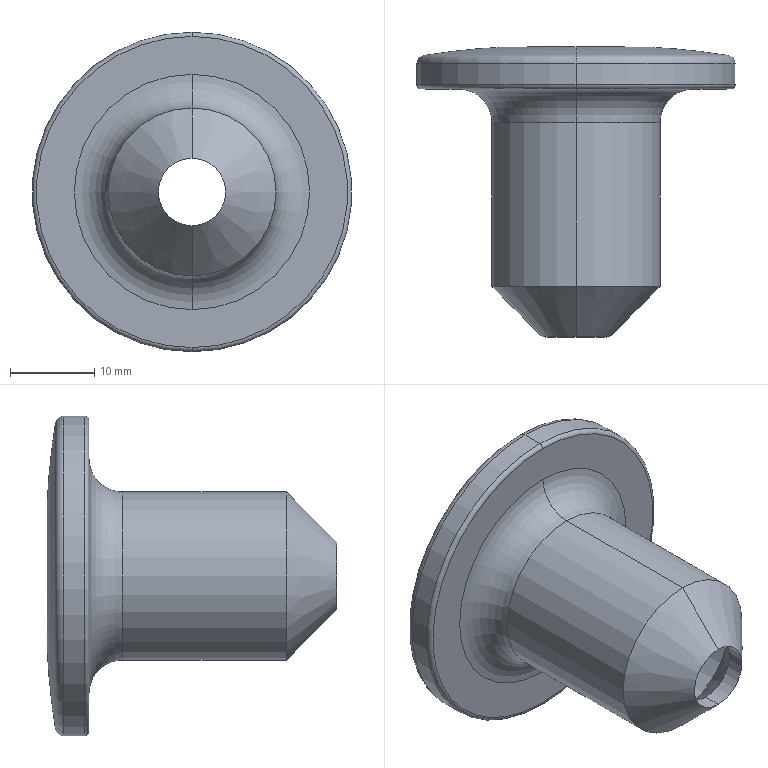Part | SolidWorks | features Cut 1, ICE 1, Revolution 1 | 1 solid | 27 faces | box 38 x 34.477 x 38 mm | volume 6932 mm3 | cylinder 12 | torus 8 | cone 4 | plane 3 | commonest cylinder face diameters 17 x4 8 x2 11 x2 20 x2 38 x2
STEP:
#1=CARTESIAN_POINT('',(0.,-17.379,-4.));
#2=VERTEX_POINT('',#1);
#3=CARTESIAN_POINT('',(0.,-17.379,4.));
#4=VERTEX_POINT('',#3);
#5=CARTESIAN_POINT('',(0.,-17.379,0.));
#6=DIRECTION('',(0.,1.,0.));
#7=DIRECTION('',(0.,0.,1.));
#8=AXIS2_PLACEMENT_3D('',#5,#6,#7);
#9=CIRCLE('',#8,4.);
#10=EDGE_CURVE('',#2,#4,#9,.T.);
#11=ORIENTED_EDGE('',*,*,#10,.T.);
#12=CARTESIAN_POINT('',(0.,-19.5,4.));
#13=VERTEX_POINT('',#12);
#14=CARTESIAN_POINT('',(0.,-10.,4.));
#15=DIRECTION('',(0.,-1.,0.));
#16=VECTOR('',#15,1000.);
#17=LINE('',#14,#16);
#18=EDGE_CURVE('',#4,#13,#17,.T.);
#19=ORIENTED_EDGE('',*,*,#18,.T.);
#20=CARTESIAN_POINT('',(0.,-19.5,-4.));
#21=VERTEX_POINT('',#20);
#22=CARTESIAN_POINT('',(0.,-19.5,0.));
#23=DIRECTION('',(0.,1.,0.));
#24=DIRECTION('',(0.,0.,1.));
#25=AXIS2_PLACEMENT_3D('',#22,#23,#24);
#26=CIRCLE('',#25,4.);
#27=EDGE_CURVE('',#21,#13,#26,.T.);
#28=ORIENTED_EDGE('',*,*,#27,.F.);
#29=CARTESIAN_POINT('',(0.,-10.,-4.));
#30=DIRECTION('',(0.,-1.,0.));
#31=VECTOR('',#30,1000.);
#32=LINE('',#29,#31);
#33=EDGE_CURVE('',#2,#21,#32,.T.);
#34=ORIENTED_EDGE('',*,*,#33,.F.);
#35=EDGE_LOOP('',(#11,#19,#28,#34));
#36=FACE_OUTER_BOUND('',#35,.T.);
#37=CARTESIAN_POINT('',(0.,-10.,0.));
#38=DIRECTION('',(0.,-1.,0.));
#39=DIRECTION('',(0.,0.,-1.));
#40=AXIS2_PLACEMENT_3D('',#37,#38,#39);
#41=CYLINDRICAL_SURFACE('',#40,4.);
#42=ADVANCED_FACE('',(#36),#41,.F.);
#43=CARTESIAN_POINT('',(0.,10.5,19.));
#44=VERTEX_POINT('',#43);
#45=CARTESIAN_POINT('',(0.,10.5,-19.));
#46=VERTEX_POINT('',#45);
#47=CARTESIAN_POINT('',(0.,10.5,0.));
#48=DIRECTION('',(0.,1.,0.));
#49=DIRECTION('',(0.,0.,1.));
#50=AXIS2_PLACEMENT_3D('',#47,#48,#49);
#51=CIRCLE('',#50,19.);
#52=EDGE_CURVE('',#44,#46,#51,.T.);
#53=ORIENTED_EDGE('',*,*,#52,.T.);
#54=CARTESIAN_POINT('',(0.,13.,-19.));
#55=VERTEX_POINT('',#54);
#56=CARTESIAN_POINT('',(0.,14.,-19.));
#57=DIRECTION('',(0.,1.,0.));
#58=VECTOR('',#57,1000.);
#59=LINE('',#56,#58);
#60=EDGE_CURVE('',#46,#55,#59,.T.);
#61=ORIENTED_EDGE('',*,*,#60,.T.);
#62=CARTESIAN_POINT('',(0.,13.,19.));
#63=VERTEX_POINT('',#62);
#64=CARTESIAN_POINT('',(0.,13.,0.));
#65=DIRECTION('',(0.,1.,0.));
#66=DIRECTION('',(0.,0.,1.));
#67=AXIS2_PLACEMENT_3D('',#64,#65,#66);
#68=CIRCLE('',#67,19.);
#69=EDGE_CURVE('',#63,#55,#68,.T.);
#70=ORIENTED_EDGE('',*,*,#69,.F.);
#71=CARTESIAN_POINT('',(0.,14.,19.));
#72=DIRECTION('',(0.,1.,0.));
#73=VECTOR('',#72,1000.);
#74=LINE('',#71,#73);
#75=EDGE_CURVE('',#44,#63,#74,.T.);
#76=ORIENTED_EDGE('',*,*,#75,.F.);
#77=EDGE_LOOP('',(#53,#61,#70,#76));
#78=FACE_OUTER_BOUND('',#77,.T.);
#79=CARTESIAN_POINT('',(0.,14.,0.));
#80=DIRECTION('',(0.,1.,0.));
#81=DIRECTION('',(0.,0.,1.));
#82=AXIS2_PLACEMENT_3D('',#79,#80,#81);
#83=CYLINDRICAL_SURFACE('',#82,19.);
#84=ADVANCED_FACE('',(#78),#83,.T.);
#85=ORIENTED_EDGE('',*,*,#69,.T.);
#86=CARTESIAN_POINT('',(0.,14.,-18.));
#87=VERTEX_POINT('',#86);
#88=CARTESIAN_POINT('',(0.,13.,-18.));
#89=DIRECTION('',(1.,0.,0.));
#90=DIRECTION('',(0.,0.,-1.));
#91=AXIS2_PLACEMENT_3D('',#88,#89,#90);
#92=CIRCLE('',#91,1.);
#93=EDGE_CURVE('',#55,#87,#92,.T.);
#94=ORIENTED_EDGE('',*,*,#93,.T.);
#95=CARTESIAN_POINT('',(0.,14.,18.));
#96=VERTEX_POINT('',#95);
#97=CARTESIAN_POINT('',(0.,14.,0.));
#98=DIRECTION('',(0.,1.,0.));
#99=DIRECTION('',(0.,0.,1.));
#100=AXIS2_PLACEMENT_3D('',#97,#98,#99);
#101=CIRCLE('',#100,18.);
#102=EDGE_CURVE('',#96,#87,#101,.T.);
#103=ORIENTED_EDGE('',*,*,#102,.F.);
#104=CARTESIAN_POINT('',(0.,13.,18.));
#105=DIRECTION('',(-1.,0.,0.));
#106=DIRECTION('',(0.,0.,1.));
#107=AXIS2_PLACEMENT_3D('',#104,#105,#106);
#108=CIRCLE('',#107,1.);
#109=EDGE_CURVE('',#63,#96,#108,.T.);
#110=ORIENTED_EDGE('',*,*,#109,.F.);
#111=EDGE_LOOP('',(#85,#94,#103,#110));
#112=FACE_OUTER_BOUND('',#111,.T.);
#113=CARTESIAN_POINT('',(0.,13.,0.));
#114=DIRECTION('',(0.,1.,0.));
#115=DIRECTION('',(0.,0.,1.));
#116=AXIS2_PLACEMENT_3D('',#113,#114,#115);
#117=TOROIDAL_SURFACE('',#116,18.,1.);
#118=ADVANCED_FACE('',(#112),#117,.T.);
#119=ORIENTED_EDGE('',*,*,#102,.T.);
#120=CARTESIAN_POINT('',(0.,14.977,-8.5));
#121=VERTEX_POINT('',#120);
#122=CARTESIAN_POINT('',(0.,-66.038,-4.966));
#123=DIRECTION('',(1.,0.,0.));
#124=DIRECTION('',(0.,0.,-1.));
#125=AXIS2_PLACEMENT_3D('',#122,#123,#124);
#126=CIRCLE('',#125,81.092);
#127=EDGE_CURVE('',#87,#121,#126,.T.);
#128=ORIENTED_EDGE('',*,*,#127,.T.);
#129=CARTESIAN_POINT('',(0.,14.977,8.5));
#130=VERTEX_POINT('',#129);
#131=CARTESIAN_POINT('',(0.,14.977,0.));
#132=DIRECTION('',(0.,1.,0.));
#133=DIRECTION('',(0.,0.,1.));
#134=AXIS2_PLACEMENT_3D('',#131,#132,#133);
#135=CIRCLE('',#134,8.5);
#136=EDGE_CURVE('',#130,#121,#135,.T.);
#137=ORIENTED_EDGE('',*,*,#136,.F.);
#138=CARTESIAN_POINT('',(0.,-66.038,4.966));
#139=DIRECTION('',(-1.,0.,0.));
#140=DIRECTION('',(0.,0.,1.));
#141=AXIS2_PLACEMENT_3D('',#138,#139,#140);
#142=CIRCLE('',#141,81.092);
#143=EDGE_CURVE('',#96,#130,#142,.T.);
#144=ORIENTED_EDGE('',*,*,#143,.F.);
#145=EDGE_LOOP('',(#119,#128,#137,#144));
#146=FACE_OUTER_BOUND('',#145,.T.);
#147=CARTESIAN_POINT('',(0.,-66.038,0.));
#148=DIRECTION('',(0.,1.,0.));
#149=DIRECTION('',(0.,0.,1.));
#150=AXIS2_PLACEMENT_3D('',#147,#148,#149);
#151=TOROIDAL_SURFACE('',#150,4.966,81.092);
#152=ADVANCED_FACE('',(#146),#151,.T.);
#153=CARTESIAN_POINT('',(0.,5.,-8.5));
#154=VERTEX_POINT('',#153);
#155=CARTESIAN_POINT('',(0.,5.,8.5));
#156=VERTEX_POINT('',#155);
#157=CARTESIAN_POINT('',(0.,5.,0.));
#158=DIRECTION('',(0.,1.,0.));
#159=DIRECTION('',(0.,0.,1.));
#160=AXIS2_PLACEMENT_3D('',#157,#158,#159);
#161=CIRCLE('',#160,8.5);
#162=EDGE_CURVE('',#154,#156,#161,.T.);
#163=ORIENTED_EDGE('',*,*,#162,.F.);
#164=CARTESIAN_POINT('',(0.,14.,-8.5));
#165=DIRECTION('',(0.,1.,0.));
#166=VECTOR('',#165,1000.);
#167=LINE('',#164,#166);
#168=EDGE_CURVE('',#154,#121,#167,.T.);
#169=ORIENTED_EDGE('',*,*,#168,.T.);
#170=CARTESIAN_POINT('',(0.,14.977,0.));
#171=DIRECTION('',(0.,1.,0.));
#172=DIRECTION('',(0.,0.,1.));
#173=AXIS2_PLACEMENT_3D('',#170,#171,#172);
#174=CIRCLE('',#173,8.5);
#175=EDGE_CURVE('',#121,#130,#174,.T.);
#176=ORIENTED_EDGE('',*,*,#175,.T.);
#177=CARTESIAN_POINT('',(0.,14.,8.5));
#178=DIRECTION('',(0.,1.,0.));
#179=VECTOR('',#178,1000.);
#180=LINE('',#177,#179);
#181=EDGE_CURVE('',#156,#130,#180,.T.);
#182=ORIENTED_EDGE('',*,*,#181,.F.);
#183=EDGE_LOOP('',(#163,#169,#176,#182));
#184=FACE_OUTER_BOUND('',#183,.T.);
#185=CARTESIAN_POINT('',(0.,14.,0.));
#186=DIRECTION('',(0.,1.,0.));
#187=DIRECTION('',(0.,0.,1.));
#188=AXIS2_PLACEMENT_3D('',#185,#186,#187);
#189=CYLINDRICAL_SURFACE('',#188,8.5);
#190=ADVANCED_FACE('',(#184),#189,.F.);
#191=CARTESIAN_POINT('',(0.,3.5,-5.5));
#192=VERTEX_POINT('',#191);
#193=CARTESIAN_POINT('',(0.,3.5,5.5));
#194=VERTEX_POINT('',#193);
#195=CARTESIAN_POINT('',(0.,3.5,0.));
#196=DIRECTION('',(0.,1.,0.));
#197=DIRECTION('',(0.,0.,1.));
#198=AXIS2_PLACEMENT_3D('',#195,#196,#197);
#199=CIRCLE('',#198,5.5);
#200=EDGE_CURVE('',#192,#194,#199,.T.);
#201=ORIENTED_EDGE('',*,*,#200,.F.);
#202=CARTESIAN_POINT('',(0.,5.,-5.5));
#203=VERTEX_POINT('',#202);
#204=CARTESIAN_POINT('',(0.,14.,-5.5));
#205=DIRECTION('',(0.,1.,0.));
#206=VECTOR('',#205,1000.);
#207=LINE('',#204,#206);
#208=EDGE_CURVE('',#192,#203,#207,.T.);
#209=ORIENTED_EDGE('',*,*,#208,.T.);
#210=CARTESIAN_POINT('',(0.,5.,5.5));
#211=VERTEX_POINT('',#210);
#212=CARTESIAN_POINT('',(0.,5.,0.));
#213=DIRECTION('',(0.,1.,0.));
#214=DIRECTION('',(0.,0.,1.));
#215=AXIS2_PLACEMENT_3D('',#212,#213,#214);
#216=CIRCLE('',#215,5.5);
#217=EDGE_CURVE('',#203,#211,#216,.T.);
#218=ORIENTED_EDGE('',*,*,#217,.T.);
#219=CARTESIAN_POINT('',(0.,14.,5.5));
#220=DIRECTION('',(0.,1.,0.));
#221=VECTOR('',#220,1000.);
#222=LINE('',#219,#221);
#223=EDGE_CURVE('',#194,#211,#222,.T.);
#224=ORIENTED_EDGE('',*,*,#223,.F.);
#225=EDGE_LOOP('',(#201,#209,#218,#224));
#226=FACE_OUTER_BOUND('',#225,.T.);
#227=CARTESIAN_POINT('',(0.,14.,0.));
#228=DIRECTION('',(0.,1.,0.));
#229=DIRECTION('',(0.,0.,1.));
#230=AXIS2_PLACEMENT_3D('',#227,#228,#229);
#231=CYLINDRICAL_SURFACE('',#230,5.5);
#232=ADVANCED_FACE('',(#226),#231,.F.);
#233=CARTESIAN_POINT('',(0.,-12.879,-8.5));
#234=VERTEX_POINT('',#233);
#235=CARTESIAN_POINT('',(0.,-12.879,8.5));
#236=VERTEX_POINT('',#235);
#237=CARTESIAN_POINT('',(0.,-12.879,0.));
#238=DIRECTION('',(0.,1.,0.));
#239=DIRECTION('',(0.,0.,1.));
#240=AXIS2_PLACEMENT_3D('',#237,#238,#239);
#241=CIRCLE('',#240,8.5);
#242=EDGE_CURVE('',#234,#236,#241,.T.);
#243=ORIENTED_EDGE('',*,*,#242,.F.);
#244=CARTESIAN_POINT('',(0.,3.5,-8.5));
#245=VERTEX_POINT('',#244);
#246=CARTESIAN_POINT('',(0.,14.,-8.5));
#247=DIRECTION('',(0.,1.,0.));
#248=VECTOR('',#247,1000.);
#249=LINE('',#246,#248);
#250=EDGE_CURVE('',#234,#245,#249,.T.);
#251=ORIENTED_EDGE('',*,*,#250,.T.);
#252=CARTESIAN_POINT('',(0.,3.5,8.5));
#253=VERTEX_POINT('',#252);
#254=CARTESIAN_POINT('',(0.,3.5,0.));
#255=DIRECTION('',(0.,1.,0.));
#256=DIRECTION('',(0.,0.,1.));
#257=AXIS2_PLACEMENT_3D('',#254,#255,#256);
#258=CIRCLE('',#257,8.5);
#259=EDGE_CURVE('',#245,#253,#258,.T.);
#260=ORIENTED_EDGE('',*,*,#259,.T.);
#261=CARTESIAN_POINT('',(0.,14.,8.5));
#262=DIRECTION('',(0.,1.,0.));
#263=VECTOR('',#262,1000.);
#264=LINE('',#261,#263);
#265=EDGE_CURVE('',#236,#253,#264,.T.);
#266=ORIENTED_EDGE('',*,*,#265,.F.);
#267=EDGE_LOOP('',(#243,#251,#260,#266));
#268=FACE_OUTER_BOUND('',#267,.T.);
#269=CARTESIAN_POINT('',(0.,14.,0.));
#270=DIRECTION('',(0.,1.,0.));
#271=DIRECTION('',(0.,0.,1.));
#272=AXIS2_PLACEMENT_3D('',#269,#270,#271);
#273=CYLINDRICAL_SURFACE('',#272,8.5);
#274=ADVANCED_FACE('',(#268),#273,.F.);
#275=ORIENTED_EDGE('',*,*,#10,.F.);
#276=CARTESIAN_POINT('',(0.,-18.5,-2.879));
#277=DIRECTION('',(0.,0.7071,-0.7071));
#278=VECTOR('',#277,1000.);
#279=LINE('',#276,#278);
#280=EDGE_CURVE('',#2,#234,#279,.T.);
#281=ORIENTED_EDGE('',*,*,#280,.T.);
#282=ORIENTED_EDGE('',*,*,#242,.T.);
#283=CARTESIAN_POINT('',(0.,-18.5,2.879));
#284=DIRECTION('',(0.,0.7071,0.7071));
#285=VECTOR('',#284,1000.);
#286=LINE('',#283,#285);
#287=EDGE_CURVE('',#4,#236,#286,.T.);
#288=ORIENTED_EDGE('',*,*,#287,.F.);
#289=EDGE_LOOP('',(#275,#281,#282,#288));
#290=FACE_OUTER_BOUND('',#289,.T.);
#291=CARTESIAN_POINT('',(0.,-18.5,0.));
#292=DIRECTION('',(0.,1.,0.));
#293=DIRECTION('',(0.,0.,1.));
#294=AXIS2_PLACEMENT_3D('',#291,#292,#293);
#295=CONICAL_SURFACE('',#294,2.879,0.7854);
#296=ADVANCED_FACE('',(#290),#295,.F.);
#297=CARTESIAN_POINT('',(0.,-19.5,0.));
#298=DIRECTION('',(0.,1.,0.));
#299=DIRECTION('',(0.,0.,1.));
#300=AXIS2_PLACEMENT_3D('',#297,#298,#299);
#301=CIRCLE('',#300,4.);
#302=EDGE_CURVE('',#13,#21,#301,.T.);
#303=ORIENTED_EDGE('',*,*,#302,.T.);
#304=CARTESIAN_POINT('',(0.,-13.5,-10.));
#305=VERTEX_POINT('',#304);
#306=CARTESIAN_POINT('',(0.,-20.,-3.5));
#307=DIRECTION('',(0.,0.7071,-0.7071));
#308=VECTOR('',#307,1000.);
#309=LINE('',#306,#308);
#310=EDGE_CURVE('',#21,#305,#309,.T.);
#311=ORIENTED_EDGE('',*,*,#310,.T.);
#312=CARTESIAN_POINT('',(0.,-13.5,10.));
#313=VERTEX_POINT('',#312);
#314=CARTESIAN_POINT('',(0.,-13.5,0.));
#315=DIRECTION('',(0.,1.,0.));
#316=DIRECTION('',(0.,0.,1.));
#317=AXIS2_PLACEMENT_3D('',#314,#315,#316);
#318=CIRCLE('',#317,10.);
#319=EDGE_CURVE('',#313,#305,#318,.T.);
#320=ORIENTED_EDGE('',*,*,#319,.F.);
#321=CARTESIAN_POINT('',(0.,-20.,3.5));
#322=DIRECTION('',(0.,0.7071,0.7071));
#323=VECTOR('',#322,1000.);
#324=LINE('',#321,#323);
#325=EDGE_CURVE('',#13,#313,#324,.T.);
#326=ORIENTED_EDGE('',*,*,#325,.F.);
#327=EDGE_LOOP('',(#303,#311,#320,#326));
#328=FACE_OUTER_BOUND('',#327,.T.);
#329=CARTESIAN_POINT('',(0.,-20.,0.));
#330=DIRECTION('',(0.,1.,0.));
#331=DIRECTION('',(0.,0.,1.));
#332=AXIS2_PLACEMENT_3D('',#329,#330,#331);
#333=CONICAL_SURFACE('',#332,3.5,0.7854);
#334=ADVANCED_FACE('',(#328),#333,.T.);
#335=ORIENTED_EDGE('',*,*,#319,.T.);
#336=CARTESIAN_POINT('',(0.,6.,-10.));
#337=VERTEX_POINT('',#336);
#338=CARTESIAN_POINT('',(0.,14.,-10.));
#339=DIRECTION('',(0.,1.,0.));
#340=VECTOR('',#339,1000.);
#341=LINE('',#338,#340);
#342=EDGE_CURVE('',#305,#337,#341,.T.);
#343=ORIENTED_EDGE('',*,*,#342,.T.);
#344=CARTESIAN_POINT('',(0.,6.,10.));
#345=VERTEX_POINT('',#344);
#346=CARTESIAN_POINT('',(0.,6.,0.));
#347=DIRECTION('',(0.,1.,0.));
#348=DIRECTION('',(0.,0.,1.));
#349=AXIS2_PLACEMENT_3D('',#346,#347,#348);
#350=CIRCLE('',#349,10.);
#351=EDGE_CURVE('',#345,#337,#350,.T.);
#352=ORIENTED_EDGE('',*,*,#351,.F.);
#353=CARTESIAN_POINT('',(0.,14.,10.));
#354=DIRECTION('',(0.,1.,0.));
#355=VECTOR('',#354,1000.);
#356=LINE('',#353,#355);
#357=EDGE_CURVE('',#313,#345,#356,.T.);
#358=ORIENTED_EDGE('',*,*,#357,.F.);
#359=EDGE_LOOP('',(#335,#343,#352,#358));
#360=FACE_OUTER_BOUND('',#359,.T.);
#361=CARTESIAN_POINT('',(0.,14.,0.));
#362=DIRECTION('',(0.,1.,0.));
#363=DIRECTION('',(0.,0.,1.));
#364=AXIS2_PLACEMENT_3D('',#361,#362,#363);
#365=CYLINDRICAL_SURFACE('',#364,10.);
#366=ADVANCED_FACE('',(#360),#365,.T.);
#367=CARTESIAN_POINT('',(0.,10.,-14.));
#368=VERTEX_POINT('',#367);
#369=CARTESIAN_POINT('',(0.,10.,14.));
#370=VERTEX_POINT('',#369);
#371=CARTESIAN_POINT('',(0.,10.,0.));
#372=DIRECTION('',(0.,1.,0.));
#373=DIRECTION('',(0.,0.,1.));
#374=AXIS2_PLACEMENT_3D('',#371,#372,#373);
#375=CIRCLE('',#374,14.);
#376=EDGE_CURVE('',#368,#370,#375,.T.);
#377=ORIENTED_EDGE('',*,*,#376,.F.);
#378=CARTESIAN_POINT('',(0.,6.,-14.));
#379=DIRECTION('',(1.,0.,0.));
#380=DIRECTION('',(0.,0.,-1.));
#381=AXIS2_PLACEMENT_3D('',#378,#379,#380);
#382=CIRCLE('',#381,4.);
#383=EDGE_CURVE('',#368,#337,#382,.T.);
#384=ORIENTED_EDGE('',*,*,#383,.T.);
#385=CARTESIAN_POINT('',(0.,6.,0.));
#386=DIRECTION('',(0.,1.,0.));
#387=DIRECTION('',(0.,0.,1.));
#388=AXIS2_PLACEMENT_3D('',#385,#386,#387);
#389=CIRCLE('',#388,10.);
#390=EDGE_CURVE('',#337,#345,#389,.T.);
#391=ORIENTED_EDGE('',*,*,#390,.T.);
#392=CARTESIAN_POINT('',(0.,6.,14.));
#393=DIRECTION('',(-1.,0.,0.));
#394=DIRECTION('',(0.,0.,1.));
#395=AXIS2_PLACEMENT_3D('',#392,#393,#394);
#396=CIRCLE('',#395,4.);
#397=EDGE_CURVE('',#370,#345,#396,.T.);
#398=ORIENTED_EDGE('',*,*,#397,.F.);
#399=EDGE_LOOP('',(#377,#384,#391,#398));
#400=FACE_OUTER_BOUND('',#399,.T.);
#401=CARTESIAN_POINT('',(0.,6.,0.));
#402=DIRECTION('',(0.,1.,0.));
#403=DIRECTION('',(0.,0.,1.));
#404=AXIS2_PLACEMENT_3D('',#401,#402,#403);
#405=TOROIDAL_SURFACE('',#404,14.,4.);
#406=ADVANCED_FACE('',(#400),#405,.F.);
#407=CARTESIAN_POINT('',(0.,10.,18.5));
#408=VERTEX_POINT('',#407);
#409=CARTESIAN_POINT('',(0.,10.,-18.5));
#410=VERTEX_POINT('',#409);
#411=CARTESIAN_POINT('',(0.,10.,0.));
#412=DIRECTION('',(0.,1.,0.));
#413=DIRECTION('',(0.,0.,1.));
#414=AXIS2_PLACEMENT_3D('',#411,#412,#413);
#415=CIRCLE('',#414,18.5);
#416=EDGE_CURVE('',#408,#410,#415,.T.);
#417=ORIENTED_EDGE('',*,*,#416,.T.);
#418=CARTESIAN_POINT('',(0.,10.5,-18.5));
#419=DIRECTION('',(1.,0.,0.));
#420=DIRECTION('',(0.,0.,-1.));
#421=AXIS2_PLACEMENT_3D('',#418,#419,#420);
#422=CIRCLE('',#421,0.5);
#423=EDGE_CURVE('',#410,#46,#422,.T.);
#424=ORIENTED_EDGE('',*,*,#423,.T.);
#425=ORIENTED_EDGE('',*,*,#52,.F.);
#426=CARTESIAN_POINT('',(0.,10.5,18.5));
#427=DIRECTION('',(-1.,0.,0.));
#428=DIRECTION('',(0.,0.,1.));
#429=AXIS2_PLACEMENT_3D('',#426,#427,#428);
#430=CIRCLE('',#429,0.5);
#431=EDGE_CURVE('',#408,#44,#430,.T.);
#432=ORIENTED_EDGE('',*,*,#431,.F.);
#433=EDGE_LOOP('',(#417,#424,#425,#432));
#434=FACE_OUTER_BOUND('',#433,.T.);
#435=CARTESIAN_POINT('',(0.,10.5,0.));
#436=DIRECTION('',(0.,1.,0.));
#437=DIRECTION('',(0.,0.,1.));
#438=AXIS2_PLACEMENT_3D('',#435,#436,#437);
#439=TOROIDAL_SURFACE('',#438,18.5,0.5);
#440=ADVANCED_FACE('',(#434),#439,.T.);
#441=ORIENTED_EDGE('',*,*,#423,.F.);
#442=CARTESIAN_POINT('',(0.,10.,0.));
#443=DIRECTION('',(0.,1.,0.));
#444=DIRECTION('',(0.,0.,1.));
#445=AXIS2_PLACEMENT_3D('',#442,#443,#444);
#446=CIRCLE('',#445,18.5);
#447=EDGE_CURVE('',#410,#408,#446,.T.);
#448=ORIENTED_EDGE('',*,*,#447,.T.);
#449=ORIENTED_EDGE('',*,*,#431,.T.);
#450=CARTESIAN_POINT('',(0.,10.5,0.));
#451=DIRECTION('',(0.,1.,0.));
#452=DIRECTION('',(0.,0.,1.));
#453=AXIS2_PLACEMENT_3D('',#450,#451,#452);
#454=CIRCLE('',#453,19.);
#455=EDGE_CURVE('',#46,#44,#454,.T.);
#456=ORIENTED_EDGE('',*,*,#455,.F.);
#457=EDGE_LOOP('',(#441,#448,#449,#456));
#458=FACE_OUTER_BOUND('',#457,.T.);
#459=CARTESIAN_POINT('',(0.,10.5,0.));
#460=DIRECTION('',(0.,1.,0.));
#461=DIRECTION('',(0.,0.,1.));
#462=AXIS2_PLACEMENT_3D('',#459,#460,#461);
#463=TOROIDAL_SURFACE('',#462,18.5,0.5);
#464=ADVANCED_FACE('',(#458),#463,.T.);
#465=ORIENTED_EDGE('',*,*,#416,.F.);
#466=ORIENTED_EDGE('',*,*,#447,.F.);
#467=EDGE_LOOP('',(#465,#466));
#468=FACE_OUTER_BOUND('',#467,.T.);
#469=CARTESIAN_POINT('',(0.,10.,0.));
#470=DIRECTION('',(0.,1.,0.));
#471=DIRECTION('',(0.,0.,1.));
#472=AXIS2_PLACEMENT_3D('',#469,#470,#471);
#473=CIRCLE('',#472,14.);
#474=EDGE_CURVE('',#370,#368,#473,.T.);
#475=ORIENTED_EDGE('',*,*,#474,.T.);
#476=ORIENTED_EDGE('',*,*,#376,.T.);
#477=EDGE_LOOP('',(#475,#476));
#478=FACE_BOUND('',#477,.T.);
#479=CARTESIAN_POINT('',(0.,10.,0.));
#480=DIRECTION('',(0.,1.,0.));
#481=DIRECTION('',(0.,0.,1.));
#482=AXIS2_PLACEMENT_3D('',#479,#480,#481);
#483=PLANE('',#482);
#484=ADVANCED_FACE('',(#468,#478),#483,.F.);
#485=ORIENTED_EDGE('',*,*,#383,.F.);
#486=ORIENTED_EDGE('',*,*,#474,.F.);
#487=ORIENTED_EDGE('',*,*,#397,.T.);
#488=ORIENTED_EDGE('',*,*,#351,.T.);
#489=EDGE_LOOP('',(#485,#486,#487,#488));
#490=FACE_OUTER_BOUND('',#489,.T.);
#491=CARTESIAN_POINT('',(0.,6.,0.));
#492=DIRECTION('',(0.,1.,0.));
#493=DIRECTION('',(0.,0.,1.));
#494=AXIS2_PLACEMENT_3D('',#491,#492,#493);
#495=TOROIDAL_SURFACE('',#494,14.,4.);
#496=ADVANCED_FACE('',(#490),#495,.F.);
#497=ORIENTED_EDGE('',*,*,#342,.F.);
#498=CARTESIAN_POINT('',(0.,-13.5,0.));
#499=DIRECTION('',(0.,1.,0.));
#500=DIRECTION('',(0.,0.,1.));
#501=AXIS2_PLACEMENT_3D('',#498,#499,#500);
#502=CIRCLE('',#501,10.);
#503=EDGE_CURVE('',#305,#313,#502,.T.);
#504=ORIENTED_EDGE('',*,*,#503,.T.);
#505=ORIENTED_EDGE('',*,*,#357,.T.);
#506=ORIENTED_EDGE('',*,*,#390,.F.);
#507=EDGE_LOOP('',(#497,#504,#505,#506));
#508=FACE_OUTER_BOUND('',#507,.T.);
#509=CARTESIAN_POINT('',(0.,14.,0.));
#510=DIRECTION('',(0.,1.,0.));
#511=DIRECTION('',(0.,0.,1.));
#512=AXIS2_PLACEMENT_3D('',#509,#510,#511);
#513=CYLINDRICAL_SURFACE('',#512,10.);
#514=ADVANCED_FACE('',(#508),#513,.T.);
#515=ORIENTED_EDGE('',*,*,#310,.F.);
#516=ORIENTED_EDGE('',*,*,#27,.T.);
#517=ORIENTED_EDGE('',*,*,#325,.T.);
#518=ORIENTED_EDGE('',*,*,#503,.F.);
#519=EDGE_LOOP('',(#515,#516,#517,#518));
#520=FACE_OUTER_BOUND('',#519,.T.);
#521=CARTESIAN_POINT('',(0.,-20.,0.));
#522=DIRECTION('',(0.,1.,0.));
#523=DIRECTION('',(0.,0.,1.));
#524=AXIS2_PLACEMENT_3D('',#521,#522,#523);
#525=CONICAL_SURFACE('',#524,3.5,0.7854);
#526=ADVANCED_FACE('',(#520),#525,.T.);
#527=ORIENTED_EDGE('',*,*,#280,.F.);
#528=CARTESIAN_POINT('',(0.,-17.379,0.));
#529=DIRECTION('',(0.,1.,0.));
#530=DIRECTION('',(0.,0.,1.));
#531=AXIS2_PLACEMENT_3D('',#528,#529,#530);
#532=CIRCLE('',#531,4.);
#533=EDGE_CURVE('',#4,#2,#532,.T.);
#534=ORIENTED_EDGE('',*,*,#533,.F.);
#535=ORIENTED_EDGE('',*,*,#287,.T.);
#536=CARTESIAN_POINT('',(0.,-12.879,0.));
#537=DIRECTION('',(0.,1.,0.));
#538=DIRECTION('',(0.,0.,1.));
#539=AXIS2_PLACEMENT_3D('',#536,#537,#538);
#540=CIRCLE('',#539,8.5);
#541=EDGE_CURVE('',#236,#234,#540,.T.);
#542=ORIENTED_EDGE('',*,*,#541,.T.);
#543=EDGE_LOOP('',(#527,#534,#535,#542));
#544=FACE_OUTER_BOUND('',#543,.T.);
#545=CARTESIAN_POINT('',(0.,-18.5,0.));
#546=DIRECTION('',(0.,1.,0.));
#547=DIRECTION('',(0.,0.,1.));
#548=AXIS2_PLACEMENT_3D('',#545,#546,#547);
#549=CONICAL_SURFACE('',#548,2.879,0.7854);
#550=ADVANCED_FACE('',(#544),#549,.F.);
#551=ORIENTED_EDGE('',*,*,#250,.F.);
#552=ORIENTED_EDGE('',*,*,#541,.F.);
#553=ORIENTED_EDGE('',*,*,#265,.T.);
#554=CARTESIAN_POINT('',(0.,3.5,0.));
#555=DIRECTION('',(0.,1.,0.));
#556=DIRECTION('',(0.,0.,1.));
#557=AXIS2_PLACEMENT_3D('',#554,#555,#556);
#558=CIRCLE('',#557,8.5);
#559=EDGE_CURVE('',#253,#245,#558,.T.);
#560=ORIENTED_EDGE('',*,*,#559,.T.);
#561=EDGE_LOOP('',(#551,#552,#553,#560));
#562=FACE_OUTER_BOUND('',#561,.T.);
#563=CARTESIAN_POINT('',(0.,14.,0.));
#564=DIRECTION('',(0.,1.,0.));
#565=DIRECTION('',(0.,0.,1.));
#566=AXIS2_PLACEMENT_3D('',#563,#564,#565);
#567=CYLINDRICAL_SURFACE('',#566,8.5);
#568=ADVANCED_FACE('',(#562),#567,.F.);
#569=ORIENTED_EDGE('',*,*,#559,.F.);
#570=ORIENTED_EDGE('',*,*,#259,.F.);
#571=EDGE_LOOP('',(#569,#570));
#572=FACE_OUTER_BOUND('',#571,.T.);
#573=CARTESIAN_POINT('',(0.,3.5,0.));
#574=DIRECTION('',(0.,1.,0.));
#575=DIRECTION('',(0.,0.,1.));
#576=AXIS2_PLACEMENT_3D('',#573,#574,#575);
#577=CIRCLE('',#576,5.5);
#578=EDGE_CURVE('',#194,#192,#577,.T.);
#579=ORIENTED_EDGE('',*,*,#578,.T.);
#580=ORIENTED_EDGE('',*,*,#200,.T.);
#581=EDGE_LOOP('',(#579,#580));
#582=FACE_BOUND('',#581,.T.);
#583=CARTESIAN_POINT('',(0.,3.5,0.));
#584=DIRECTION('',(0.,1.,0.));
#585=DIRECTION('',(0.,0.,1.));
#586=AXIS2_PLACEMENT_3D('',#583,#584,#585);
#587=PLANE('',#586);
#588=ADVANCED_FACE('',(#572,#582),#587,.F.);
#589=ORIENTED_EDGE('',*,*,#208,.F.);
#590=ORIENTED_EDGE('',*,*,#578,.F.);
#591=ORIENTED_EDGE('',*,*,#223,.T.);
#592=CARTESIAN_POINT('',(0.,5.,0.));
#593=DIRECTION('',(0.,1.,0.));
#594=DIRECTION('',(0.,0.,1.));
#595=AXIS2_PLACEMENT_3D('',#592,#593,#594);
#596=CIRCLE('',#595,5.5);
#597=EDGE_CURVE('',#211,#203,#596,.T.);
#598=ORIENTED_EDGE('',*,*,#597,.T.);
#599=EDGE_LOOP('',(#589,#590,#591,#598));
#600=FACE_OUTER_BOUND('',#599,.T.);
#601=CARTESIAN_POINT('',(0.,14.,0.));
#602=DIRECTION('',(0.,1.,0.));
#603=DIRECTION('',(0.,0.,1.));
#604=AXIS2_PLACEMENT_3D('',#601,#602,#603);
#605=CYLINDRICAL_SURFACE('',#604,5.5);
#606=ADVANCED_FACE('',(#600),#605,.F.);
#607=ORIENTED_EDGE('',*,*,#597,.F.);
#608=ORIENTED_EDGE('',*,*,#217,.F.);
#609=EDGE_LOOP('',(#607,#608));
#610=FACE_BOUND('',#609,.T.);
#611=CARTESIAN_POINT('',(0.,5.,0.));
#612=DIRECTION('',(0.,1.,0.));
#613=DIRECTION('',(0.,0.,1.));
#614=AXIS2_PLACEMENT_3D('',#611,#612,#613);
#615=CIRCLE('',#614,8.5);
#616=EDGE_CURVE('',#156,#154,#615,.T.);
#617=ORIENTED_EDGE('',*,*,#616,.T.);
#618=ORIENTED_EDGE('',*,*,#162,.T.);
#619=EDGE_LOOP('',(#617,#618));
#620=FACE_OUTER_BOUND('',#619,.T.);
#621=CARTESIAN_POINT('',(0.,5.,0.));
#622=DIRECTION('',(0.,-1.,0.));
#623=DIRECTION('',(0.,0.,-1.));
#624=AXIS2_PLACEMENT_3D('',#621,#622,#623);
#625=PLANE('',#624);
#626=ADVANCED_FACE('',(#610,#620),#625,.F.);
#627=ORIENTED_EDGE('',*,*,#168,.F.);
#628=ORIENTED_EDGE('',*,*,#616,.F.);
#629=ORIENTED_EDGE('',*,*,#181,.T.);
#630=ORIENTED_EDGE('',*,*,#136,.T.);
#631=EDGE_LOOP('',(#627,#628,#629,#630));
#632=FACE_OUTER_BOUND('',#631,.T.);
#633=CARTESIAN_POINT('',(0.,14.,0.));
#634=DIRECTION('',(0.,1.,0.));
#635=DIRECTION('',(0.,0.,1.));
#636=AXIS2_PLACEMENT_3D('',#633,#634,#635);
#637=CYLINDRICAL_SURFACE('',#636,8.5);
#638=ADVANCED_FACE('',(#632),#637,.F.);
#639=ORIENTED_EDGE('',*,*,#127,.F.);
#640=CARTESIAN_POINT('',(0.,14.,0.));
#641=DIRECTION('',(0.,1.,0.));
#642=DIRECTION('',(0.,0.,1.));
#643=AXIS2_PLACEMENT_3D('',#640,#641,#642);
#644=CIRCLE('',#643,18.);
#645=EDGE_CURVE('',#87,#96,#644,.T.);
#646=ORIENTED_EDGE('',*,*,#645,.T.);
#647=ORIENTED_EDGE('',*,*,#143,.T.);
#648=ORIENTED_EDGE('',*,*,#175,.F.);
#649=EDGE_LOOP('',(#639,#646,#647,#648));
#650=FACE_OUTER_BOUND('',#649,.T.);
#651=CARTESIAN_POINT('',(0.,-66.038,0.));
#652=DIRECTION('',(0.,1.,0.));
#653=DIRECTION('',(0.,0.,1.));
#654=AXIS2_PLACEMENT_3D('',#651,#652,#653);
#655=TOROIDAL_SURFACE('',#654,4.966,81.092);
#656=ADVANCED_FACE('',(#650),#655,.T.);
#657=ORIENTED_EDGE('',*,*,#93,.F.);
#658=CARTESIAN_POINT('',(0.,13.,0.));
#659=DIRECTION('',(0.,1.,0.));
#660=DIRECTION('',(0.,0.,1.));
#661=AXIS2_PLACEMENT_3D('',#658,#659,#660);
#662=CIRCLE('',#661,19.);
#663=EDGE_CURVE('',#55,#63,#662,.T.);
#664=ORIENTED_EDGE('',*,*,#663,.T.);
#665=ORIENTED_EDGE('',*,*,#109,.T.);
#666=ORIENTED_EDGE('',*,*,#645,.F.);
#667=EDGE_LOOP('',(#657,#664,#665,#666));
#668=FACE_OUTER_BOUND('',#667,.T.);
#669=CARTESIAN_POINT('',(0.,13.,0.));
#670=DIRECTION('',(0.,1.,0.));
#671=DIRECTION('',(0.,0.,1.));
#672=AXIS2_PLACEMENT_3D('',#669,#670,#671);
#673=TOROIDAL_SURFACE('',#672,18.,1.);
#674=ADVANCED_FACE('',(#668),#673,.T.);
#675=ORIENTED_EDGE('',*,*,#60,.F.);
#676=ORIENTED_EDGE('',*,*,#455,.T.);
#677=ORIENTED_EDGE('',*,*,#75,.T.);
#678=ORIENTED_EDGE('',*,*,#663,.F.);
#679=EDGE_LOOP('',(#675,#676,#677,#678));
#680=FACE_OUTER_BOUND('',#679,.T.);
#681=CARTESIAN_POINT('',(0.,14.,0.));
#682=DIRECTION('',(0.,1.,0.));
#683=DIRECTION('',(0.,0.,1.));
#684=AXIS2_PLACEMENT_3D('',#681,#682,#683);
#685=CYLINDRICAL_SURFACE('',#684,19.);
#686=ADVANCED_FACE('',(#680),#685,.T.);
#687=ORIENTED_EDGE('',*,*,#18,.F.);
#688=ORIENTED_EDGE('',*,*,#533,.T.);
#689=ORIENTED_EDGE('',*,*,#33,.T.);
#690=ORIENTED_EDGE('',*,*,#302,.F.);
#691=EDGE_LOOP('',(#687,#688,#689,#690));
#692=FACE_OUTER_BOUND('',#691,.T.);
#693=CARTESIAN_POINT('',(0.,-10.,0.));
#694=DIRECTION('',(0.,-1.,0.));
#695=DIRECTION('',(0.,0.,-1.));
#696=AXIS2_PLACEMENT_3D('',#693,#694,#695);
#697=CYLINDRICAL_SURFACE('',#696,4.);
#698=ADVANCED_FACE('',(#692),#697,.F.);
#699=CLOSED_SHELL('',(#42,#84,#118,#152,#190,#232,#274,#296,#334,#366,#406,#440,#464,#484,#496,#514,#526,#550,#568,#588,#606,#626,#638,#656,#674,#686,#698));
#700=MANIFOLD_SOLID_BREP('',#699);
#701=CARTESIAN_POINT('',(0.,0.,0.));
#702=DIRECTION('',(0.,0.,1.));
#703=DIRECTION('',(1.,0.,0.));
#704=AXIS2_PLACEMENT_3D('',#701,#702,#703);
#705=(LENGTH_UNIT()NAMED_UNIT(*)SI_UNIT(.MILLI.,.METRE.));
#706=UNCERTAINTY_MEASURE_WITH_UNIT(LENGTH_MEASURE(0.00001),#705,'','');
#707=(NAMED_UNIT(*)PLANE_ANGLE_UNIT()SI_UNIT($,.RADIAN.));
#708=(NAMED_UNIT(*)SI_UNIT($,.STERADIAN.)SOLID_ANGLE_UNIT());
#709=(GEOMETRIC_REPRESENTATION_CONTEXT(3)GLOBAL_UNCERTAINTY_ASSIGNED_CONTEXT((#706))GLOBAL_UNIT_ASSIGNED_CONTEXT((#705,#707,#708))REPRESENTATION_CONTEXT('',''));
#710=ADVANCED_BREP_SHAPE_REPRESENTATION('',(#700,#704),#709);